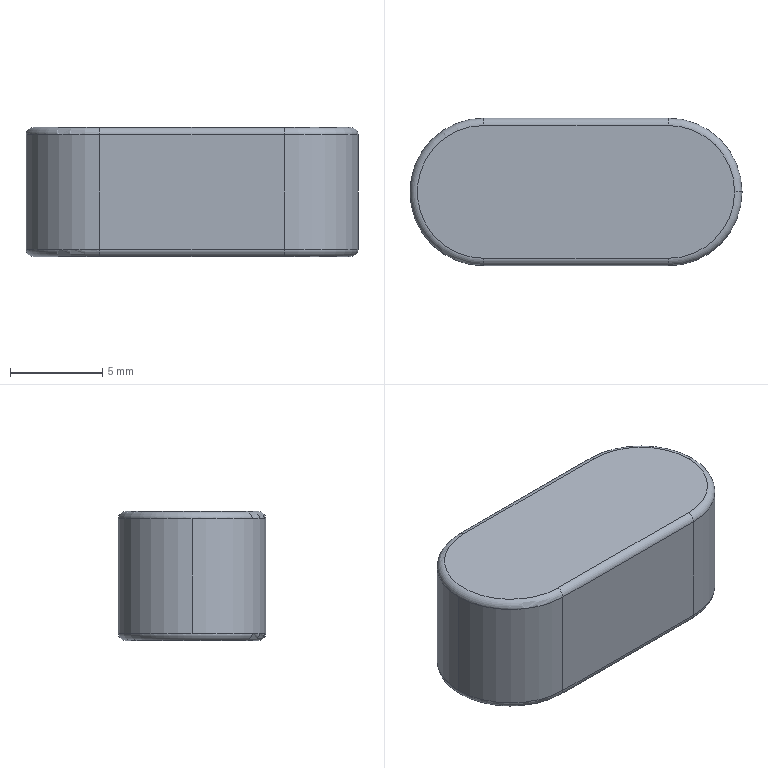Part | SolidWorks | features Extrusion 1, Fillet 1 | 1 solid | 17 faces | box 18 x 8 x 7 mm | volume 908.798 mm3 | cylinder 7 | torus 6 | plane 4 | commonest cylinder face diameters 0.8 x4 8 x3
STEP:
#1=CARTESIAN_POINT('',(8.6,0.,0.));
#2=VERTEX_POINT('',#1);
#3=CARTESIAN_POINT('',(5.,-3.6,0.));
#4=VERTEX_POINT('',#3);
#5=CARTESIAN_POINT('',(5.,0.,0.));
#6=DIRECTION('',(0.,0.,-1.));
#7=DIRECTION('',(1.,0.,0.));
#8=AXIS2_PLACEMENT_3D('',#5,#6,#7);
#9=CIRCLE('',#8,3.6);
#10=EDGE_CURVE('',#2,#4,#9,.T.);
#11=ORIENTED_EDGE('',*,*,#10,.F.);
#12=CARTESIAN_POINT('',(9.,0.,0.4));
#13=VERTEX_POINT('',#12);
#14=CARTESIAN_POINT('',(8.6,0.,0.4));
#15=DIRECTION('',(0.,-1.,0.));
#16=DIRECTION('',(0.,0.,-1.));
#17=AXIS2_PLACEMENT_3D('',#14,#15,#16);
#18=CIRCLE('',#17,0.4);
#19=EDGE_CURVE('',#2,#13,#18,.T.);
#20=ORIENTED_EDGE('',*,*,#19,.T.);
#21=CARTESIAN_POINT('',(5.,-4.,0.4));
#22=VERTEX_POINT('',#21);
#23=CARTESIAN_POINT('',(5.,0.,0.4));
#24=DIRECTION('',(0.,0.,1.));
#25=DIRECTION('',(1.,0.,0.));
#26=AXIS2_PLACEMENT_3D('',#23,#24,#25);
#27=CIRCLE('',#26,4.);
#28=EDGE_CURVE('',#22,#13,#27,.T.);
#29=ORIENTED_EDGE('',*,*,#28,.F.);
#30=CARTESIAN_POINT('',(5.,-3.6,0.4));
#31=DIRECTION('',(1.,0.,0.));
#32=DIRECTION('',(0.,0.,-1.));
#33=AXIS2_PLACEMENT_3D('',#30,#31,#32);
#34=CIRCLE('',#33,0.4);
#35=EDGE_CURVE('',#22,#4,#34,.T.);
#36=ORIENTED_EDGE('',*,*,#35,.T.);
#37=EDGE_LOOP('',(#11,#20,#29,#36));
#38=FACE_OUTER_BOUND('',#37,.T.);
#39=CARTESIAN_POINT('',(5.,0.,0.4));
#40=DIRECTION('',(0.,0.,1.));
#41=DIRECTION('',(1.,0.,0.));
#42=AXIS2_PLACEMENT_3D('',#39,#40,#41);
#43=TOROIDAL_SURFACE('',#42,3.6,0.4);
#44=ADVANCED_FACE('',(#38),#43,.T.);
#45=CARTESIAN_POINT('',(9.,0.,6.6));
#46=VERTEX_POINT('',#45);
#47=CARTESIAN_POINT('',(5.,-4.,6.6));
#48=VERTEX_POINT('',#47);
#49=CARTESIAN_POINT('',(5.,0.,6.6));
#50=DIRECTION('',(0.,0.,-1.));
#51=DIRECTION('',(1.,0.,0.));
#52=AXIS2_PLACEMENT_3D('',#49,#50,#51);
#53=CIRCLE('',#52,4.);
#54=EDGE_CURVE('',#46,#48,#53,.T.);
#55=ORIENTED_EDGE('',*,*,#54,.F.);
#56=CARTESIAN_POINT('',(8.6,0.,7.));
#57=VERTEX_POINT('',#56);
#58=CARTESIAN_POINT('',(8.6,0.,6.6));
#59=DIRECTION('',(0.,-1.,0.));
#60=DIRECTION('',(0.,0.,-1.));
#61=AXIS2_PLACEMENT_3D('',#58,#59,#60);
#62=CIRCLE('',#61,0.4);
#63=EDGE_CURVE('',#46,#57,#62,.T.);
#64=ORIENTED_EDGE('',*,*,#63,.T.);
#65=CARTESIAN_POINT('',(5.,-3.6,7.));
#66=VERTEX_POINT('',#65);
#67=CARTESIAN_POINT('',(5.,0.,7.));
#68=DIRECTION('',(0.,0.,1.));
#69=DIRECTION('',(1.,0.,0.));
#70=AXIS2_PLACEMENT_3D('',#67,#68,#69);
#71=CIRCLE('',#70,3.6);
#72=EDGE_CURVE('',#66,#57,#71,.T.);
#73=ORIENTED_EDGE('',*,*,#72,.F.);
#74=CARTESIAN_POINT('',(5.,-3.6,6.6));
#75=DIRECTION('',(1.,0.,0.));
#76=DIRECTION('',(0.,0.,-1.));
#77=AXIS2_PLACEMENT_3D('',#74,#75,#76);
#78=CIRCLE('',#77,0.4);
#79=EDGE_CURVE('',#66,#48,#78,.T.);
#80=ORIENTED_EDGE('',*,*,#79,.T.);
#81=EDGE_LOOP('',(#55,#64,#73,#80));
#82=FACE_OUTER_BOUND('',#81,.T.);
#83=CARTESIAN_POINT('',(5.,0.,6.6));
#84=DIRECTION('',(0.,0.,1.));
#85=DIRECTION('',(1.,0.,0.));
#86=AXIS2_PLACEMENT_3D('',#83,#84,#85);
#87=TOROIDAL_SURFACE('',#86,3.6,0.4);
#88=ADVANCED_FACE('',(#82),#87,.T.);
#89=CARTESIAN_POINT('',(-5.,-4.,6.6));
#90=VERTEX_POINT('',#89);
#91=CARTESIAN_POINT('',(-9.,0.,6.6));
#92=VERTEX_POINT('',#91);
#93=CARTESIAN_POINT('',(-5.,0.,6.6));
#94=DIRECTION('',(0.,0.,-1.));
#95=DIRECTION('',(1.,0.,0.));
#96=AXIS2_PLACEMENT_3D('',#93,#94,#95);
#97=CIRCLE('',#96,4.);
#98=EDGE_CURVE('',#90,#92,#97,.T.);
#99=ORIENTED_EDGE('',*,*,#98,.T.);
#100=CARTESIAN_POINT('',(-9.,0.,0.4));
#101=VERTEX_POINT('',#100);
#102=CARTESIAN_POINT('',(-9.,0.,7.));
#103=DIRECTION('',(0.,0.,-1.));
#104=VECTOR('',#103,1000.);
#105=LINE('',#102,#104);
#106=EDGE_CURVE('',#92,#101,#105,.T.);
#107=ORIENTED_EDGE('',*,*,#106,.T.);
#108=CARTESIAN_POINT('',(-5.,-4.,0.4));
#109=VERTEX_POINT('',#108);
#110=CARTESIAN_POINT('',(-5.,0.,0.4));
#111=DIRECTION('',(0.,0.,1.));
#112=DIRECTION('',(1.,0.,0.));
#113=AXIS2_PLACEMENT_3D('',#110,#111,#112);
#114=CIRCLE('',#113,4.);
#115=EDGE_CURVE('',#101,#109,#114,.T.);
#116=ORIENTED_EDGE('',*,*,#115,.T.);
#117=CARTESIAN_POINT('',(-5.,-4.,7.));
#118=DIRECTION('',(0.,0.,-1.));
#119=VECTOR('',#118,1000.);
#120=LINE('',#117,#119);
#121=EDGE_CURVE('',#90,#109,#120,.T.);
#122=ORIENTED_EDGE('',*,*,#121,.F.);
#123=EDGE_LOOP('',(#99,#107,#116,#122));
#124=FACE_OUTER_BOUND('',#123,.T.);
#125=CARTESIAN_POINT('',(-5.,0.,7.));
#126=DIRECTION('',(0.,0.,-1.));
#127=DIRECTION('',(-1.,0.,0.));
#128=AXIS2_PLACEMENT_3D('',#125,#126,#127);
#129=CYLINDRICAL_SURFACE('',#128,4.);
#130=ADVANCED_FACE('',(#124),#129,.T.);
#131=ORIENTED_EDGE('',*,*,#106,.F.);
#132=CARTESIAN_POINT('',(-5.,4.,6.6));
#133=VERTEX_POINT('',#132);
#134=CARTESIAN_POINT('',(-5.,0.,6.6));
#135=DIRECTION('',(0.,0.,-1.));
#136=DIRECTION('',(1.,0.,0.));
#137=AXIS2_PLACEMENT_3D('',#134,#135,#136);
#138=CIRCLE('',#137,4.);
#139=EDGE_CURVE('',#92,#133,#138,.T.);
#140=ORIENTED_EDGE('',*,*,#139,.T.);
#141=CARTESIAN_POINT('',(-5.,4.,0.4));
#142=VERTEX_POINT('',#141);
#143=CARTESIAN_POINT('',(-5.,4.,7.));
#144=DIRECTION('',(0.,0.,-1.));
#145=VECTOR('',#144,1000.);
#146=LINE('',#143,#145);
#147=EDGE_CURVE('',#133,#142,#146,.T.);
#148=ORIENTED_EDGE('',*,*,#147,.T.);
#149=CARTESIAN_POINT('',(-5.,0.,0.4));
#150=DIRECTION('',(0.,0.,1.));
#151=DIRECTION('',(1.,0.,0.));
#152=AXIS2_PLACEMENT_3D('',#149,#150,#151);
#153=CIRCLE('',#152,4.);
#154=EDGE_CURVE('',#142,#101,#153,.T.);
#155=ORIENTED_EDGE('',*,*,#154,.T.);
#156=EDGE_LOOP('',(#131,#140,#148,#155));
#157=FACE_OUTER_BOUND('',#156,.T.);
#158=CARTESIAN_POINT('',(-5.,0.,7.));
#159=DIRECTION('',(0.,0.,-1.));
#160=DIRECTION('',(-1.,0.,0.));
#161=AXIS2_PLACEMENT_3D('',#158,#159,#160);
#162=CYLINDRICAL_SURFACE('',#161,4.);
#163=ADVANCED_FACE('',(#157),#162,.T.);
#164=CARTESIAN_POINT('',(5.,-4.,7.));
#165=DIRECTION('',(0.,0.,-1.));
#166=VECTOR('',#165,1000.);
#167=LINE('',#164,#166);
#168=EDGE_CURVE('',#48,#22,#167,.T.);
#169=ORIENTED_EDGE('',*,*,#168,.F.);
#170=CARTESIAN_POINT('',(-5.,-4.,6.6));
#171=DIRECTION('',(-1.,0.,0.));
#172=VECTOR('',#171,1000.);
#173=LINE('',#170,#172);
#174=EDGE_CURVE('',#48,#90,#173,.T.);
#175=ORIENTED_EDGE('',*,*,#174,.T.);
#176=ORIENTED_EDGE('',*,*,#121,.T.);
#177=CARTESIAN_POINT('',(-5.,-4.,0.4));
#178=DIRECTION('',(1.,0.,0.));
#179=VECTOR('',#178,1000.);
#180=LINE('',#177,#179);
#181=EDGE_CURVE('',#109,#22,#180,.T.);
#182=ORIENTED_EDGE('',*,*,#181,.T.);
#183=EDGE_LOOP('',(#169,#175,#176,#182));
#184=FACE_OUTER_BOUND('',#183,.T.);
#185=CARTESIAN_POINT('',(-5.,-4.,7.));
#186=DIRECTION('',(0.,1.,0.));
#187=DIRECTION('',(-1.,0.,0.));
#188=AXIS2_PLACEMENT_3D('',#185,#186,#187);
#189=PLANE('',#188);
#190=ADVANCED_FACE('',(#184),#189,.F.);
#191=CARTESIAN_POINT('',(5.,4.,6.6));
#192=VERTEX_POINT('',#191);
#193=CARTESIAN_POINT('',(5.,4.,0.4));
#194=VERTEX_POINT('',#193);
#195=CARTESIAN_POINT('',(5.,4.,7.));
#196=DIRECTION('',(0.,0.,-1.));
#197=VECTOR('',#196,1000.);
#198=LINE('',#195,#197);
#199=EDGE_CURVE('',#192,#194,#198,.T.);
#200=ORIENTED_EDGE('',*,*,#199,.F.);
#201=CARTESIAN_POINT('',(5.,0.,6.6));
#202=DIRECTION('',(0.,0.,-1.));
#203=DIRECTION('',(1.,0.,0.));
#204=AXIS2_PLACEMENT_3D('',#201,#202,#203);
#205=CIRCLE('',#204,4.);
#206=EDGE_CURVE('',#192,#46,#205,.T.);
#207=ORIENTED_EDGE('',*,*,#206,.T.);
#208=ORIENTED_EDGE('',*,*,#54,.T.);
#209=ORIENTED_EDGE('',*,*,#168,.T.);
#210=ORIENTED_EDGE('',*,*,#28,.T.);
#211=CARTESIAN_POINT('',(5.,0.,0.4));
#212=DIRECTION('',(0.,0.,1.));
#213=DIRECTION('',(1.,0.,0.));
#214=AXIS2_PLACEMENT_3D('',#211,#212,#213);
#215=CIRCLE('',#214,4.);
#216=EDGE_CURVE('',#13,#194,#215,.T.);
#217=ORIENTED_EDGE('',*,*,#216,.T.);
#218=EDGE_LOOP('',(#200,#207,#208,#209,#210,#217));
#219=FACE_OUTER_BOUND('',#218,.T.);
#220=CARTESIAN_POINT('',(5.,0.,7.));
#221=DIRECTION('',(0.,0.,-1.));
#222=DIRECTION('',(-1.,0.,0.));
#223=AXIS2_PLACEMENT_3D('',#220,#221,#222);
#224=CYLINDRICAL_SURFACE('',#223,4.);
#225=ADVANCED_FACE('',(#219),#224,.T.);
#226=ORIENTED_EDGE('',*,*,#147,.F.);
#227=CARTESIAN_POINT('',(5.,4.,6.6));
#228=DIRECTION('',(1.,0.,0.));
#229=VECTOR('',#228,1000.);
#230=LINE('',#227,#229);
#231=EDGE_CURVE('',#133,#192,#230,.T.);
#232=ORIENTED_EDGE('',*,*,#231,.T.);
#233=ORIENTED_EDGE('',*,*,#199,.T.);
#234=CARTESIAN_POINT('',(-5.,4.,0.4));
#235=DIRECTION('',(-1.,0.,0.));
#236=VECTOR('',#235,1000.);
#237=LINE('',#234,#236);
#238=EDGE_CURVE('',#194,#142,#237,.T.);
#239=ORIENTED_EDGE('',*,*,#238,.T.);
#240=EDGE_LOOP('',(#226,#232,#233,#239));
#241=FACE_OUTER_BOUND('',#240,.T.);
#242=CARTESIAN_POINT('',(-5.,4.,7.));
#243=DIRECTION('',(0.,-1.,0.));
#244=DIRECTION('',(1.,0.,0.));
#245=AXIS2_PLACEMENT_3D('',#242,#243,#244);
#246=PLANE('',#245);
#247=ADVANCED_FACE('',(#241),#246,.F.);
#248=CARTESIAN_POINT('',(-5.,-3.6,7.));
#249=VERTEX_POINT('',#248);
#250=CARTESIAN_POINT('',(5.,-3.6,7.));
#251=DIRECTION('',(1.,0.,0.));
#252=VECTOR('',#251,1000.);
#253=LINE('',#250,#252);
#254=EDGE_CURVE('',#249,#66,#253,.T.);
#255=ORIENTED_EDGE('',*,*,#254,.T.);
#256=ORIENTED_EDGE('',*,*,#72,.T.);
#257=CARTESIAN_POINT('',(5.,3.6,7.));
#258=VERTEX_POINT('',#257);
#259=CARTESIAN_POINT('',(5.,0.,7.));
#260=DIRECTION('',(0.,0.,1.));
#261=DIRECTION('',(1.,0.,0.));
#262=AXIS2_PLACEMENT_3D('',#259,#260,#261);
#263=CIRCLE('',#262,3.6);
#264=EDGE_CURVE('',#57,#258,#263,.T.);
#265=ORIENTED_EDGE('',*,*,#264,.T.);
#266=CARTESIAN_POINT('',(-5.,3.6,7.));
#267=VERTEX_POINT('',#266);
#268=CARTESIAN_POINT('',(-5.,3.6,7.));
#269=DIRECTION('',(-1.,0.,0.));
#270=VECTOR('',#269,1000.);
#271=LINE('',#268,#270);
#272=EDGE_CURVE('',#258,#267,#271,.T.);
#273=ORIENTED_EDGE('',*,*,#272,.T.);
#274=CARTESIAN_POINT('',(-5.,0.,7.));
#275=DIRECTION('',(0.,0.,1.));
#276=DIRECTION('',(1.,0.,0.));
#277=AXIS2_PLACEMENT_3D('',#274,#275,#276);
#278=CIRCLE('',#277,3.6);
#279=EDGE_CURVE('',#267,#249,#278,.T.);
#280=ORIENTED_EDGE('',*,*,#279,.T.);
#281=EDGE_LOOP('',(#255,#256,#265,#273,#280));
#282=FACE_OUTER_BOUND('',#281,.T.);
#283=CARTESIAN_POINT('',(-5.,0.,7.));
#284=DIRECTION('',(0.,0.,1.));
#285=DIRECTION('',(1.,0.,0.));
#286=AXIS2_PLACEMENT_3D('',#283,#284,#285);
#287=PLANE('',#286);
#288=ADVANCED_FACE('',(#282),#287,.T.);
#289=CARTESIAN_POINT('',(-5.,3.6,0.));
#290=VERTEX_POINT('',#289);
#291=CARTESIAN_POINT('',(5.,3.6,0.));
#292=VERTEX_POINT('',#291);
#293=CARTESIAN_POINT('',(-5.,3.6,0.));
#294=DIRECTION('',(1.,0.,0.));
#295=VECTOR('',#294,1000.);
#296=LINE('',#293,#295);
#297=EDGE_CURVE('',#290,#292,#296,.T.);
#298=ORIENTED_EDGE('',*,*,#297,.T.);
#299=CARTESIAN_POINT('',(5.,0.,0.));
#300=DIRECTION('',(0.,0.,-1.));
#301=DIRECTION('',(1.,0.,0.));
#302=AXIS2_PLACEMENT_3D('',#299,#300,#301);
#303=CIRCLE('',#302,3.6);
#304=EDGE_CURVE('',#292,#2,#303,.T.);
#305=ORIENTED_EDGE('',*,*,#304,.T.);
#306=ORIENTED_EDGE('',*,*,#10,.T.);
#307=CARTESIAN_POINT('',(-5.,-3.6,0.));
#308=VERTEX_POINT('',#307);
#309=CARTESIAN_POINT('',(-5.,-3.6,0.));
#310=DIRECTION('',(-1.,0.,0.));
#311=VECTOR('',#310,1000.);
#312=LINE('',#309,#311);
#313=EDGE_CURVE('',#4,#308,#312,.T.);
#314=ORIENTED_EDGE('',*,*,#313,.T.);
#315=CARTESIAN_POINT('',(-5.,0.,0.));
#316=DIRECTION('',(0.,0.,-1.));
#317=DIRECTION('',(1.,0.,0.));
#318=AXIS2_PLACEMENT_3D('',#315,#316,#317);
#319=CIRCLE('',#318,3.6);
#320=EDGE_CURVE('',#308,#290,#319,.T.);
#321=ORIENTED_EDGE('',*,*,#320,.T.);
#322=EDGE_LOOP('',(#298,#305,#306,#314,#321));
#323=FACE_OUTER_BOUND('',#322,.T.);
#324=CARTESIAN_POINT('',(-5.,0.,0.));
#325=DIRECTION('',(0.,0.,1.));
#326=DIRECTION('',(1.,0.,0.));
#327=AXIS2_PLACEMENT_3D('',#324,#325,#326);
#328=PLANE('',#327);
#329=ADVANCED_FACE('',(#323),#328,.F.);
#330=CARTESIAN_POINT('',(-5.,3.6,6.6));
#331=DIRECTION('',(1.,0.,0.));
#332=DIRECTION('',(0.,0.,-1.));
#333=AXIS2_PLACEMENT_3D('',#330,#331,#332);
#334=CIRCLE('',#333,0.4);
#335=EDGE_CURVE('',#133,#267,#334,.T.);
#336=ORIENTED_EDGE('',*,*,#335,.F.);
#337=ORIENTED_EDGE('',*,*,#139,.F.);
#338=ORIENTED_EDGE('',*,*,#98,.F.);
#339=CARTESIAN_POINT('',(-5.,-3.6,6.6));
#340=DIRECTION('',(1.,0.,0.));
#341=DIRECTION('',(0.,0.,-1.));
#342=AXIS2_PLACEMENT_3D('',#339,#340,#341);
#343=CIRCLE('',#342,0.4);
#344=EDGE_CURVE('',#249,#90,#343,.T.);
#345=ORIENTED_EDGE('',*,*,#344,.F.);
#346=ORIENTED_EDGE('',*,*,#279,.F.);
#347=EDGE_LOOP('',(#336,#337,#338,#345,#346));
#348=FACE_OUTER_BOUND('',#347,.T.);
#349=CARTESIAN_POINT('',(-5.,0.,6.6));
#350=DIRECTION('',(0.,0.,1.));
#351=DIRECTION('',(1.,0.,0.));
#352=AXIS2_PLACEMENT_3D('',#349,#350,#351);
#353=TOROIDAL_SURFACE('',#352,3.6,0.4);
#354=ADVANCED_FACE('',(#348),#353,.T.);
#355=ORIENTED_EDGE('',*,*,#344,.T.);
#356=ORIENTED_EDGE('',*,*,#174,.F.);
#357=ORIENTED_EDGE('',*,*,#79,.F.);
#358=ORIENTED_EDGE('',*,*,#254,.F.);
#359=EDGE_LOOP('',(#355,#356,#357,#358));
#360=FACE_OUTER_BOUND('',#359,.T.);
#361=CARTESIAN_POINT('',(-5.,-3.6,6.6));
#362=DIRECTION('',(-1.,0.,0.));
#363=DIRECTION('',(0.,-1.,0.));
#364=AXIS2_PLACEMENT_3D('',#361,#362,#363);
#365=CYLINDRICAL_SURFACE('',#364,0.4);
#366=ADVANCED_FACE('',(#360),#365,.T.);
#367=ORIENTED_EDGE('',*,*,#335,.T.);
#368=ORIENTED_EDGE('',*,*,#272,.F.);
#369=CARTESIAN_POINT('',(5.,3.6,6.6));
#370=DIRECTION('',(1.,0.,0.));
#371=DIRECTION('',(0.,0.,-1.));
#372=AXIS2_PLACEMENT_3D('',#369,#370,#371);
#373=CIRCLE('',#372,0.4);
#374=EDGE_CURVE('',#192,#258,#373,.T.);
#375=ORIENTED_EDGE('',*,*,#374,.F.);
#376=ORIENTED_EDGE('',*,*,#231,.F.);
#377=EDGE_LOOP('',(#367,#368,#375,#376));
#378=FACE_OUTER_BOUND('',#377,.T.);
#379=CARTESIAN_POINT('',(-5.,3.6,6.6));
#380=DIRECTION('',(1.,0.,0.));
#381=DIRECTION('',(0.,1.,0.));
#382=AXIS2_PLACEMENT_3D('',#379,#380,#381);
#383=CYLINDRICAL_SURFACE('',#382,0.4);
#384=ADVANCED_FACE('',(#378),#383,.T.);
#385=ORIENTED_EDGE('',*,*,#63,.F.);
#386=ORIENTED_EDGE('',*,*,#206,.F.);
#387=ORIENTED_EDGE('',*,*,#374,.T.);
#388=ORIENTED_EDGE('',*,*,#264,.F.);
#389=EDGE_LOOP('',(#385,#386,#387,#388));
#390=FACE_OUTER_BOUND('',#389,.T.);
#391=CARTESIAN_POINT('',(5.,0.,6.6));
#392=DIRECTION('',(0.,0.,1.));
#393=DIRECTION('',(1.,0.,0.));
#394=AXIS2_PLACEMENT_3D('',#391,#392,#393);
#395=TOROIDAL_SURFACE('',#394,3.6,0.4);
#396=ADVANCED_FACE('',(#390),#395,.T.);
#397=CARTESIAN_POINT('',(-5.,3.6,0.4));
#398=DIRECTION('',(1.,0.,0.));
#399=DIRECTION('',(0.,0.,-1.));
#400=AXIS2_PLACEMENT_3D('',#397,#398,#399);
#401=CIRCLE('',#400,0.4);
#402=EDGE_CURVE('',#290,#142,#401,.T.);
#403=ORIENTED_EDGE('',*,*,#402,.F.);
#404=ORIENTED_EDGE('',*,*,#320,.F.);
#405=CARTESIAN_POINT('',(-5.,-3.6,0.4));
#406=DIRECTION('',(1.,0.,0.));
#407=DIRECTION('',(0.,0.,-1.));
#408=AXIS2_PLACEMENT_3D('',#405,#406,#407);
#409=CIRCLE('',#408,0.4);
#410=EDGE_CURVE('',#109,#308,#409,.T.);
#411=ORIENTED_EDGE('',*,*,#410,.F.);
#412=ORIENTED_EDGE('',*,*,#115,.F.);
#413=ORIENTED_EDGE('',*,*,#154,.F.);
#414=EDGE_LOOP('',(#403,#404,#411,#412,#413));
#415=FACE_OUTER_BOUND('',#414,.T.);
#416=CARTESIAN_POINT('',(-5.,0.,0.4));
#417=DIRECTION('',(0.,0.,1.));
#418=DIRECTION('',(1.,0.,0.));
#419=AXIS2_PLACEMENT_3D('',#416,#417,#418);
#420=TOROIDAL_SURFACE('',#419,3.6,0.4);
#421=ADVANCED_FACE('',(#415),#420,.T.);
#422=ORIENTED_EDGE('',*,*,#410,.T.);
#423=ORIENTED_EDGE('',*,*,#313,.F.);
#424=ORIENTED_EDGE('',*,*,#35,.F.);
#425=ORIENTED_EDGE('',*,*,#181,.F.);
#426=EDGE_LOOP('',(#422,#423,#424,#425));
#427=FACE_OUTER_BOUND('',#426,.T.);
#428=CARTESIAN_POINT('',(-5.,-3.6,0.4));
#429=DIRECTION('',(1.,0.,0.));
#430=DIRECTION('',(0.,1.,0.));
#431=AXIS2_PLACEMENT_3D('',#428,#429,#430);
#432=CYLINDRICAL_SURFACE('',#431,0.4);
#433=ADVANCED_FACE('',(#427),#432,.T.);
#434=ORIENTED_EDGE('',*,*,#402,.T.);
#435=ORIENTED_EDGE('',*,*,#238,.F.);
#436=CARTESIAN_POINT('',(5.,3.6,0.4));
#437=DIRECTION('',(1.,0.,0.));
#438=DIRECTION('',(0.,0.,-1.));
#439=AXIS2_PLACEMENT_3D('',#436,#437,#438);
#440=CIRCLE('',#439,0.4);
#441=EDGE_CURVE('',#292,#194,#440,.T.);
#442=ORIENTED_EDGE('',*,*,#441,.F.);
#443=ORIENTED_EDGE('',*,*,#297,.F.);
#444=EDGE_LOOP('',(#434,#435,#442,#443));
#445=FACE_OUTER_BOUND('',#444,.T.);
#446=CARTESIAN_POINT('',(-5.,3.6,0.4));
#447=DIRECTION('',(-1.,0.,0.));
#448=DIRECTION('',(0.,-1.,0.));
#449=AXIS2_PLACEMENT_3D('',#446,#447,#448);
#450=CYLINDRICAL_SURFACE('',#449,0.4);
#451=ADVANCED_FACE('',(#445),#450,.T.);
#452=ORIENTED_EDGE('',*,*,#19,.F.);
#453=ORIENTED_EDGE('',*,*,#304,.F.);
#454=ORIENTED_EDGE('',*,*,#441,.T.);
#455=ORIENTED_EDGE('',*,*,#216,.F.);
#456=EDGE_LOOP('',(#452,#453,#454,#455));
#457=FACE_OUTER_BOUND('',#456,.T.);
#458=CARTESIAN_POINT('',(5.,0.,0.4));
#459=DIRECTION('',(0.,0.,1.));
#460=DIRECTION('',(1.,0.,0.));
#461=AXIS2_PLACEMENT_3D('',#458,#459,#460);
#462=TOROIDAL_SURFACE('',#461,3.6,0.4);
#463=ADVANCED_FACE('',(#457),#462,.T.);
#464=CLOSED_SHELL('',(#44,#88,#130,#163,#190,#225,#247,#288,#329,#354,#366,#384,#396,#421,#433,#451,#463));
#465=MANIFOLD_SOLID_BREP('',#464);
#466=CARTESIAN_POINT('',(0.,0.,0.));
#467=DIRECTION('',(0.,0.,1.));
#468=DIRECTION('',(1.,0.,0.));
#469=AXIS2_PLACEMENT_3D('',#466,#467,#468);
#470=(LENGTH_UNIT()NAMED_UNIT(*)SI_UNIT(.MILLI.,.METRE.));
#471=UNCERTAINTY_MEASURE_WITH_UNIT(LENGTH_MEASURE(0.00001),#470,'','');
#472=(NAMED_UNIT(*)PLANE_ANGLE_UNIT()SI_UNIT($,.RADIAN.));
#473=(NAMED_UNIT(*)SI_UNIT($,.STERADIAN.)SOLID_ANGLE_UNIT());
#474=(GEOMETRIC_REPRESENTATION_CONTEXT(3)GLOBAL_UNCERTAINTY_ASSIGNED_CONTEXT((#471))GLOBAL_UNIT_ASSIGNED_CONTEXT((#470,#472,#473))REPRESENTATION_CONTEXT('',''));
#475=ADVANCED_BREP_SHAPE_REPRESENTATION('',(#465,#469),#474);